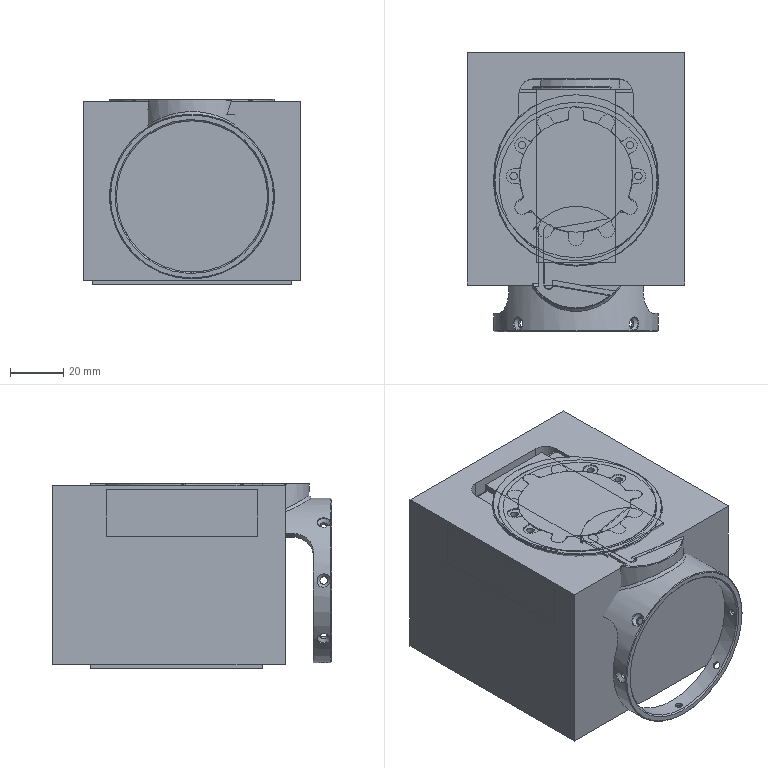NC program | NX | posted with a generic post | part box 82 x 105.2 x 70 mm
Whole program:
N10 G17 G21 G94 G90
(VARIABLE_CONTOUR_COPY_2_COPY_1_COPY_1 , TOOL : 45度燕尾刀D6)
N12 T09 M6
N14 G53
N16 G17 G0 G90 X20.986 Y-19.675 B0. C0. S12000 M3
N18 G43 Z10. H9
N20 Z-0.71
N22 G94 G1 X15.077 Y-20.717 F3000.
N24 X-8.274 Y-24.834
N26 Y-24.818 Z-0.753
N28 X15.064 Y-20.703
N30 X15.047 Y-20.686 Z-0.807
N32 X-8.274 Y-24.798
N34 Y-24.783 Z-0.851
N36 X15.034 Y-20.673
N38 X15.018 Y-20.656 Z-0.905
N40 X-8.274 Y-24.763
N42 Y-24.747 Z-0.948
N44 X15.005 Y-20.642
N46 X14.989 Y-20.625 Z-1.002
N48 X-8.274 Y-24.727
N50 Y-24.712 Z-1.045
N52 X14.976 Y-20.612
N54 X14.96 Y-20.595 Z-1.099
N56 X-8.274 Y-24.692
N58 Y-24.676 Z-1.142
N60 X14.947 Y-20.582
N62 X14.93 Y-20.565 Z-1.196
N64 X-8.274 Y-24.656
N66 Y-24.64 Z-1.239
N68 X14.917 Y-20.551
N70 X14.901 Y-20.534 Z-1.293
N72 X-8.274 Y-24.621
N74 Y-24.605 Z-1.337
N76 X14.888 Y-20.521
N78 X14.872 Y-20.504 Z-1.391
N80 X-8.274 Y-24.585
N82 Y-24.569 Z-1.434
N84 X14.859 Y-20.49
N86 X14.842 Y-20.474 Z-1.488
N88 X-8.274 Y-24.55
N90 Y-24.534 Z-1.531
N92 X14.829 Y-20.46
N94 X14.813 Y-20.443 Z-1.585
N96 X-8.274 Y-24.514
N98 Y-24.498 Z-1.628
N100 X14.8 Y-20.43
N102 X14.784 Y-20.413 Z-1.682
N104 X-8.274 Y-24.479
N106 Y-24.463 Z-1.725
N108 X14.771 Y-20.399
N110 X14.754 Y-20.382 Z-1.779
N112 X-8.274 Y-24.443
N114 Y-24.427 Z-1.823
N116 X14.741 Y-20.369
N118 X14.725 Y-20.352 Z-1.877
N120 X-8.274 Y-24.408
N122 Y-24.392 Z-1.92
N124 X14.712 Y-20.339
N126 X14.696 Y-20.322 Z-1.974
N128 X-8.274 Y-24.372
N130 Y-24.356 Z-2.017
N132 X14.683 Y-20.308
N134 X14.667 Y-20.291 Z-2.071
N136 X-8.274 Y-24.336
N138 Y-24.321 Z-2.114
N140 X14.654 Y-20.278
N142 X14.637 Y-20.261 Z-2.168
N144 X-8.274 Y-24.301
N146 Y-24.285 Z-2.211
N148 X14.624 Y-20.248
N150 X14.608 Y-20.231 Z-2.265
N152 X-8.274 Y-24.265
N154 Y-24.25 Z-2.309
N156 X14.595 Y-20.217
N158 X14.579 Y-20.2 Z-2.363
N160 X-8.274 Y-24.23
N162 Y-24.214 Z-2.406
N164 X14.566 Y-20.187
N166 X14.549 Y-20.17 Z-2.46
N168 X-8.274 Y-24.194
N170 Y-24.179 Z-2.503
N172 X14.536 Y-20.156
N174 X14.52 Y-20.14 Z-2.557
N176 X-8.274 Y-24.159
N178 Y-24.143 Z-2.6
N180 X14.507 Y-20.126
N182 X14.491 Y-20.109 Z-2.654
N184 X-8.274 Y-24.123
N186 Y-24.107 Z-2.697
N188 X14.478 Y-20.096
N190 X14.462 Y-20.079 Z-2.751
N192 X-8.274 Y-24.088
N194 Y-24.072 Z-2.795
N196 X14.449 Y-20.065
N198 X14.432 Y-20.048 Z-2.849
N200 X-8.274 Y-24.052
N202 Y-24.036 Z-2.892
N204 X14.419 Y-20.035
N206 X14.403 Y-20.018 Z-2.946
N208 X-8.274 Y-24.017
N210 Y-24.001 Z-2.989
N212 X14.39 Y-20.005
N214 X14.374 Y-19.988 Z-3.043
N216 X-8.274 Y-23.981
N218 Y-23.965 Z-3.086
N220 X14.361 Y-19.974
N222 X14.344 Y-19.957 Z-3.14
N224 X-8.274 Y-23.946
N226 Y-23.93 Z-3.183
N228 X14.331 Y-19.944
N230 X14.315 Y-19.927 Z-3.237
N232 X-8.274 Y-23.91
N234 Y-23.894 Z-3.281
N236 X14.302 Y-19.913
N238 X14.286 Y-19.897 Z-3.335
N240 X-8.274 Y-23.875
N242 Y-23.859 Z-3.378
N244 X14.273 Y-19.883
N246 X14.256 Y-19.866 Z-3.432
N248 X-8.274 Y-23.839
N250 Y-23.823 Z-3.475
N252 X14.243 Y-19.853
N254 X14.227 Y-19.836 Z-3.529
N256 X-8.274 Y-23.803
N258 Y-23.788 Z-3.572
N260 X14.214 Y-19.822
N262 X14.198 Y-19.806 Z-3.626
N264 X-8.274 Y-23.768
N266 Y-23.752 Z-3.669
N268 X14.185 Y-19.792
N270 X14.169 Y-19.775 Z-3.723
N272 X-8.274 Y-23.732
N274 Y-23.717 Z-3.767
N276 X14.156 Y-19.762
N278 X14.139 Y-19.745 Z-3.821
N280 X-8.274 Y-23.697
N282 Y-23.681 Z-3.864
N284 X14.126 Y-19.731
N286 X14.11 Y-19.714 Z-3.918
N288 X-8.274 Y-23.661
N290 Y-23.646 Z-3.961
N292 X14.097 Y-19.701
N294 X14.081 Y-19.684 Z-4.015
N296 X-8.274 Y-23.626
N298 Y-23.61 Z-4.058
N300 X14.068 Y-19.671
N302 X14.051 Y-19.654 Z-4.112
N304 X-8.274 Y-23.59
N306 Y-23.575 Z-4.155
N308 X14.038 Y-19.64
N310 X14.022 Y-19.623 Z-4.209
N312 X-8.274 Y-23.555
N314 Y-23.539 Z-4.253
N316 X14.009 Y-19.61
N318 X13.993 Y-19.593 Z-4.307
N320 X-8.274 Y-23.519
N322 Y-23.503 Z-4.35
N324 X13.98 Y-19.579
N326 X13.964 Y-19.563 Z-4.404
N328 X-8.274 Y-23.484
N330 Y-23.468 Z-4.447
N332 X13.951 Y-19.549
N334 X13.934 Y-19.532 Z-4.501
N336 X-8.274 Y-23.448
N338 Y-23.432 Z-4.544
N340 X13.921 Y-19.519
N342 X13.905 Y-19.502 Z-4.598
N344 X-8.274 Y-23.413
N346 Y-23.397 Z-4.641
N348 X13.892 Y-19.488
N350 X13.876 Y-19.471 Z-4.695
N352 X-8.274 Y-23.377
N354 Y-23.361 Z-4.739
N356 X13.863 Y-19.458
N358 X13.846 Y-19.441 Z-4.793
N360 X-8.274 Y-23.342
N362 Y-23.326 Z-4.836
N364 X13.833 Y-19.428
N366 X13.817 Y-19.411 Z-4.89
N368 X-8.274 Y-23.306
N370 Y-23.29 Z-4.933
N372 X13.804 Y-19.397
N374 X13.788 Y-19.38 Z-4.987
N376 X-8.274 Y-23.271
N378 Y-23.255 Z-5.03
N380 X13.775 Y-19.367
N382 X13.758 Y-19.35 Z-5.084
N384 X-8.274 Y-23.235
N386 Y-23.219 Z-5.127
N388 X13.745 Y-19.337
N390 X13.729 Y-19.32 Z-5.181
N392 X-8.274 Y-23.199
N394 Y-23.184 Z-5.225
N396 X13.716 Y-19.306
N398 X13.7 Y-19.289 Z-5.279
N400 X-8.274 Y-23.164
N402 Y-23.148 Z-5.322
N404 X13.687 Y-19.276
N406 X13.671 Y-19.259 Z-5.376
N408 X-8.274 Y-23.128
N410 Y-23.113 Z-5.419
N412 X13.658 Y-19.245
N414 X13.641 Y-19.229 Z-5.473
N416 X-8.274 Y-23.093
N418 Y-23.077 Z-5.516
N420 X13.628 Y-19.215
N422 X13.612 Y-19.198 Z-5.57
N424 X-8.274 Y-23.057
N426 Y-23.042 Z-5.613
N428 X13.599 Y-19.185
N430 X13.583 Y-19.168 Z-5.667
N432 X-8.274 Y-23.022
N434 Y-23.006 Z-5.71
N436 X13.57 Y-19.154
N438 X19.479 Y-18.113
N440 G0 Z10.
(VARIABLE_CONTOUR_COPY_2_COPY_1_COPY_1_COPY , TOOL : 45度燕尾刀D6)
N442 X21.15 Y-41.354
N444 Z-0.71
N446 G1 X15.241 Y-40.313
N448 X-8.11 Y-36.195
N450 Y-36.215 Z-0.764
N452 X15.225 Y-40.329
N454 X15.212 Y-40.343 Z-0.807
N456 X-8.11 Y-36.231
N458 Y-36.25 Z-0.861
N460 X15.195 Y-40.36
N462 X15.182 Y-40.373 Z-0.905
N464 X-8.11 Y-36.266
N466 Y-36.286 Z-0.959
N468 X15.166 Y-40.39
N470 X15.153 Y-40.403 Z-1.002
N472 X-8.11 Y-36.302
N474 Y-36.321 Z-1.056
N476 X15.136 Y-40.42
N478 X15.123 Y-40.434 Z-1.099
N480 X-8.11 Y-36.337
N482 Y-36.357 Z-1.153
N484 X15.107 Y-40.451
N486 X15.094 Y-40.464 Z-1.196
N488 X-8.111 Y-36.373
N490 Y-36.392 Z-1.25
N492 X15.077 Y-40.481
N494 X15.064 Y-40.494 Z-1.293
N496 X-8.111 Y-36.408
N498 Y-36.428 Z-1.347
N500 X15.048 Y-40.511
N502 X15.035 Y-40.525 Z-1.391
N504 X-8.111 Y-36.444
N506 Y-36.463 Z-1.445
N508 X15.018 Y-40.542
N510 X15.005 Y-40.555 Z-1.488
N512 X-8.111 Y-36.479
N514 Y-36.499 Z-1.542
N516 X14.989 Y-40.572
N518 X14.976 Y-40.585 Z-1.585
N520 X-8.111 Y-36.515
N522 X-8.112 Y-36.534 Z-1.639
N524 X14.959 Y-40.602
N526 X14.946 Y-40.616 Z-1.682
N528 X-8.112 Y-36.55
N530 Y-36.57 Z-1.736
N532 X14.93 Y-40.633
N534 X14.917 Y-40.646 Z-1.779
N536 X-8.112 Y-36.586
N538 Y-36.605 Z-1.833
N540 X14.9 Y-40.663
N542 X14.887 Y-40.676 Z-1.877
N544 X-8.112 Y-36.621
N546 Y-36.641 Z-1.931
N548 X14.871 Y-40.693
N550 X14.858 Y-40.707 Z-1.974
N552 X-8.112 Y-36.657
N554 Y-36.676 Z-2.028
N556 X14.841 Y-40.724
N558 X14.828 Y-40.737 Z-2.071
N560 X-8.112 Y-36.692
N562 X-8.113 Y-36.712 Z-2.125
N564 X14.812 Y-40.754
N566 X14.799 Y-40.767 Z-2.168
N568 X-8.113 Y-36.728
N570 Y-36.747 Z-2.222
N572 X14.782 Y-40.784
N574 X14.769 Y-40.798 Z-2.265
N576 X-8.113 Y-36.763
N578 Y-36.783 Z-2.319
N580 X14.753 Y-40.815
N582 X14.74 Y-40.828 Z-2.363
N584 X-8.113 Y-36.799
N586 Y-36.818 Z-2.417
N588 X14.723 Y-40.845
N590 X14.71 Y-40.858 Z-2.46
N592 X-8.113 Y-36.834
N594 Y-36.854 Z-2.514
N596 X14.694 Y-40.875
N598 X14.681 Y-40.889 Z-2.557
N600 X-8.113 Y-36.87
N602 X-8.114 Y-36.889 Z-2.611
N604 X14.664 Y-40.906
N606 X14.651 Y-40.919 Z-2.654
N608 X-8.114 Y-36.905
N610 Y-36.925 Z-2.708
N612 X14.635 Y-40.936
N614 X14.622 Y-40.949 Z-2.751
N616 X-8.114 Y-36.941
N618 Y-36.96 Z-2.805
N620 X14.605 Y-40.966
N622 X14.592 Y-40.98 Z-2.849
N624 X-8.114 Y-36.976
N626 Y-36.996 Z-2.903
N628 X14.576 Y-40.997
N630 X14.563 Y-41.01 Z-2.946
N632 X-8.114 Y-37.012
N634 Y-37.031 Z-3.
N636 X14.546 Y-41.027
N638 X14.533 Y-41.04 Z-3.043
N640 X-8.115 Y-37.047
N642 Y-37.067 Z-3.097
N644 X14.517 Y-41.057
N646 X14.504 Y-41.071 Z-3.14
N648 X-8.115 Y-37.083
N650 Y-37.102 Z-3.194
N652 X14.487 Y-41.088
N654 X14.474 Y-41.101 Z-3.237
N656 X-8.115 Y-37.118
N658 Y-37.138 Z-3.291
N660 X14.458 Y-41.118
N662 X14.445 Y-41.131 Z-3.335
N664 X-8.115 Y-37.153
N666 Y-37.173 Z-3.389
N668 X14.428 Y-41.148
N670 X14.415 Y-41.162 Z-3.432
N672 X-8.115 Y-37.189
N674 Y-37.209 Z-3.486
N676 X14.399 Y-41.179
N678 X14.386 Y-41.192 Z-3.529
N680 X-8.116 Y-37.224
N682 Y-37.244 Z-3.583
N684 X14.369 Y-41.209
N686 X14.356 Y-41.222 Z-3.626
N688 X-8.116 Y-37.26
N690 Y-37.28 Z-3.68
N692 X14.34 Y-41.239
N694 X14.327 Y-41.253 Z-3.723
N696 X-8.116 Y-37.295
N698 Y-37.315 Z-3.777
N700 X14.31 Y-41.27
N702 X14.297 Y-41.283 Z-3.821
N704 X-8.116 Y-37.331
N706 Y-37.351 Z-3.875
N708 X14.281 Y-41.3
N710 X14.268 Y-41.313 Z-3.918
N712 X-8.116 Y-37.366
N714 Y-37.386 Z-3.972
N716 X14.251 Y-41.33
N718 X14.238 Y-41.344 Z-4.015
N720 X-8.117 Y-37.402
N722 Y-37.422 Z-4.069
N724 X14.222 Y-41.361
N726 X14.209 Y-41.374 Z-4.112
N728 X-8.117 Y-37.437
N730 Y-37.457 Z-4.166
N732 X14.192 Y-41.391
N734 X14.179 Y-41.404 Z-4.209
N736 X-8.117 Y-37.473
N738 Y-37.493 Z-4.263
N740 X14.163 Y-41.421
N742 X14.15 Y-41.435 Z-4.307
N744 X-8.117 Y-37.508
N746 Y-37.528 Z-4.361
N748 X14.133 Y-41.452
N750 X14.12 Y-41.465 Z-4.404
N752 X-8.117 Y-37.544
N754 X-8.118 Y-37.564 Z-4.458
N756 X14.104 Y-41.482
N758 X14.091 Y-41.495 Z-4.501
N760 X-8.118 Y-37.579
N762 Y-37.599 Z-4.555
N764 X14.074 Y-41.512
N766 X14.061 Y-41.526 Z-4.598
N768 X-8.118 Y-37.615
N770 Y-37.635 Z-4.652
N772 X14.045 Y-41.543
N774 X14.032 Y-41.556 Z-4.695
N776 X-8.118 Y-37.65
N778 Y-37.67 Z-4.749
N780 X14.015 Y-41.573
N782 X14.002 Y-41.586 Z-4.793
N784 X-8.118 Y-37.686
N786 Y-37.706 Z-4.847
N788 X13.986 Y-41.603
N790 X13.973 Y-41.617 Z-4.89
N792 X-8.118 Y-37.721
N794 X-8.119 Y-37.741 Z-4.944
N796 X13.956 Y-41.634
N798 X13.943 Y-41.647 Z-4.987
N800 X-8.119 Y-37.757
N802 Y-37.777 Z-5.041
N804 X13.927 Y-41.664
N806 X13.914 Y-41.677 Z-5.084
N808 X-8.119 Y-37.792
N810 Y-37.812 Z-5.138
N812 X13.897 Y-41.694
N814 X13.884 Y-41.708 Z-5.181
N816 X-8.119 Y-37.828
N818 Y-37.848 Z-5.235
N820 X13.868 Y-41.725
N822 X13.855 Y-41.738 Z-5.279
N824 X-8.119 Y-37.863
N826 Y-37.883 Z-5.333
N828 X13.838 Y-41.755
N830 X13.825 Y-41.768 Z-5.376
N832 X-8.119 Y-37.899
N834 X-8.12 Y-37.919 Z-5.43
N836 X13.809 Y-41.785
N838 X13.796 Y-41.799 Z-5.473
N840 X-8.12 Y-37.934
N842 Y-37.954 Z-5.527
N844 X13.779 Y-41.816
N846 X13.766 Y-41.829 Z-5.57
N848 X-8.12 Y-37.97
N850 Y-37.99 Z-5.624
N852 X13.75 Y-41.846
N854 X13.737 Y-41.859 Z-5.667
N856 X-8.12 Y-38.005
N858 Y-38.021 Z-5.71
N860 X13.724 Y-41.873
N862 X19.633 Y-42.915
N864 G0 Z10.
N866 M5
N868 M2